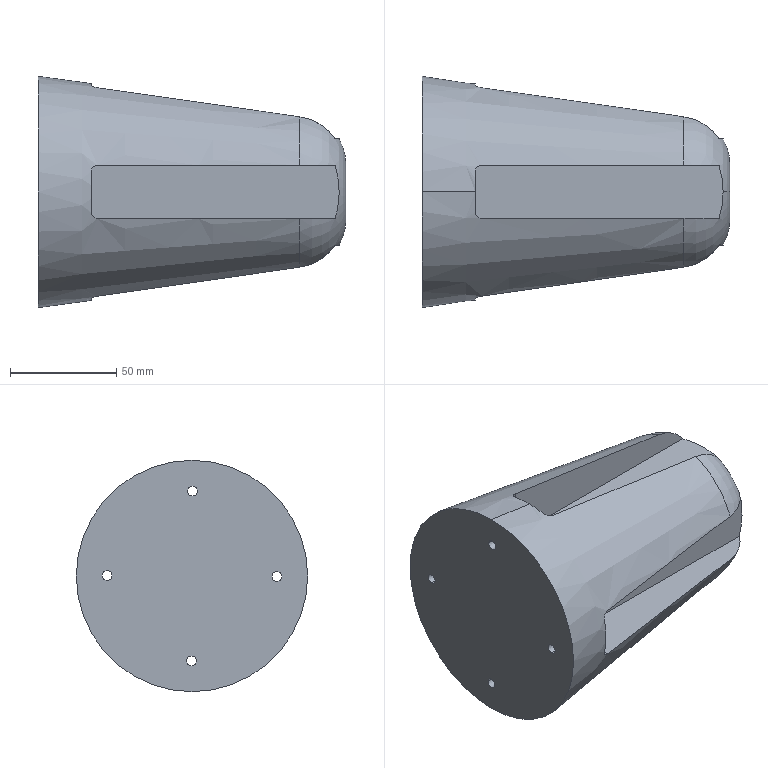Part | SolidWorks | features BaseBody 1 | 1 solid | 50 faces | box 145 x 109 x 109 mm | volume 700128 mm3 | cylinder 24 | plane 22 | torus 2 | cone 2 | commonest cylinder face diameters 4.5 x8 6 x8 8 x8